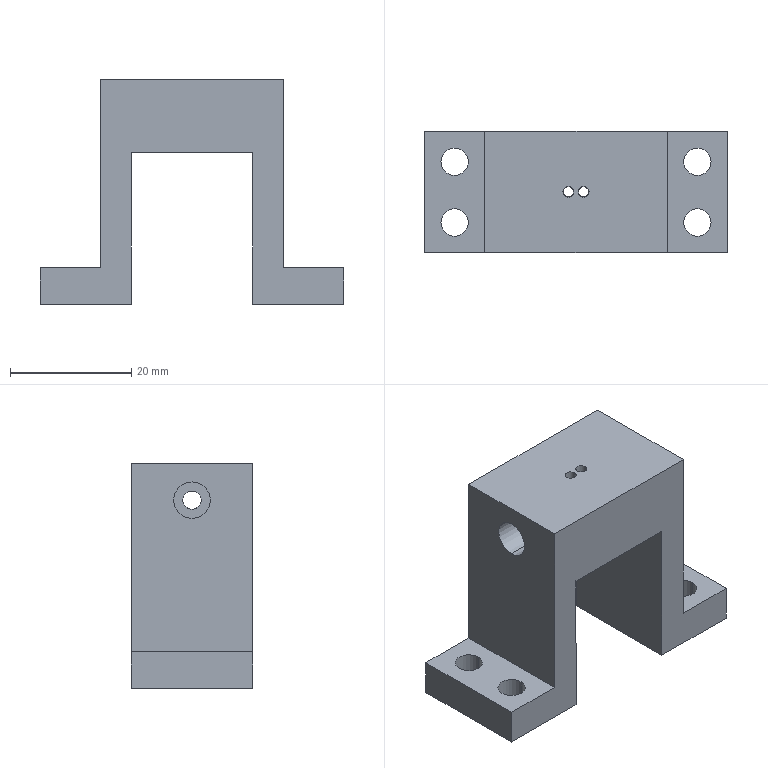Part | STEP file | X77-08304 | 1 solid | 44 faces | box 50 x 20 x 37 mm | volume 13752 mm3 | cylinder 26 | plane 18 | commonest cylinder face diameters 1.68 x8 4.5 x8 1.8 x4 6 x4 3 x2